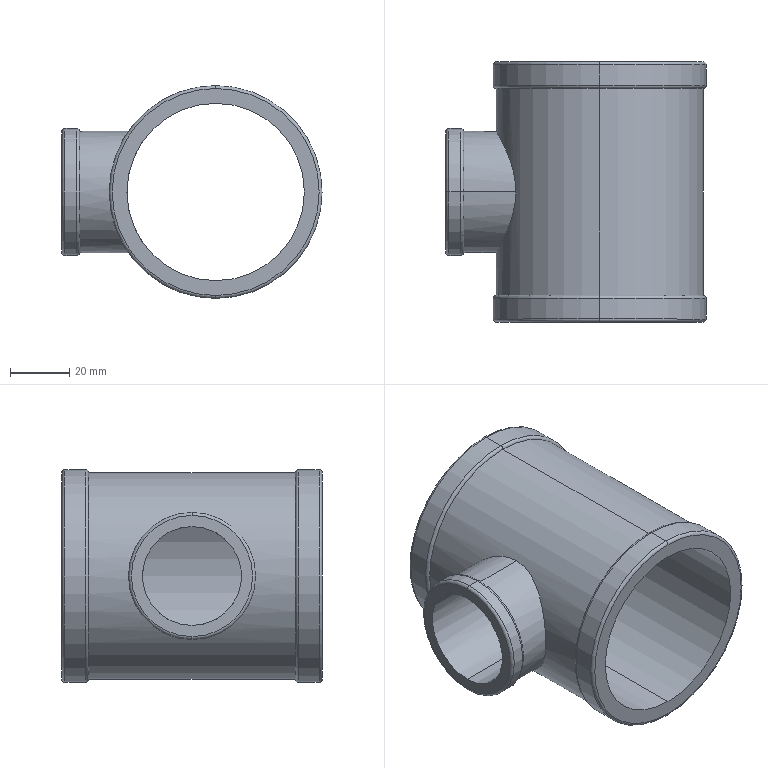Part | SolidWorks | features BossThin 3, Cut 2, Revolution 2, Fillet 1 | 1 solid | 29 faces | box 88 x 88 x 72 mm | volume 98463 mm3 | cylinder 14 | torus 12 | plane 3 | commonest cylinder face diameters 72 x4 33.5 x2 41 x2 43 x2 60 x2 70 x2
STEP:
#1=CARTESIAN_POINT('',(-51.,0.,-21.5));
#2=VERTEX_POINT('',#1);
#3=CARTESIAN_POINT('',(-51.,0.,21.5));
#4=VERTEX_POINT('',#3);
#5=CARTESIAN_POINT('',(-51.,0.,0.));
#6=DIRECTION('',(1.,0.,0.));
#7=DIRECTION('',(0.,0.,1.));
#8=AXIS2_PLACEMENT_3D('',#5,#6,#7);
#9=CIRCLE('',#8,21.5);
#10=EDGE_CURVE('',#2,#4,#9,.T.);
#11=ORIENTED_EDGE('',*,*,#10,.F.);
#12=CARTESIAN_POINT('',(-52.,0.,-20.5));
#13=VERTEX_POINT('',#12);
#14=CARTESIAN_POINT('',(-51.,0.,-20.5));
#15=DIRECTION('',(0.,1.,0.));
#16=DIRECTION('',(0.,0.,1.));
#17=AXIS2_PLACEMENT_3D('',#14,#15,#16);
#18=CIRCLE('',#17,1.);
#19=EDGE_CURVE('',#2,#13,#18,.T.);
#20=ORIENTED_EDGE('',*,*,#19,.T.);
#21=CARTESIAN_POINT('',(-52.,0.,20.5));
#22=VERTEX_POINT('',#21);
#23=CARTESIAN_POINT('',(-52.,0.,0.));
#24=DIRECTION('',(-1.,0.,0.));
#25=DIRECTION('',(0.,0.,1.));
#26=AXIS2_PLACEMENT_3D('',#23,#24,#25);
#27=CIRCLE('',#26,20.5);
#28=EDGE_CURVE('',#22,#13,#27,.T.);
#29=ORIENTED_EDGE('',*,*,#28,.F.);
#30=CARTESIAN_POINT('',(-51.,0.,20.5));
#31=DIRECTION('',(0.,-1.,0.));
#32=DIRECTION('',(0.,0.,-1.));
#33=AXIS2_PLACEMENT_3D('',#30,#31,#32);
#34=CIRCLE('',#33,1.);
#35=EDGE_CURVE('',#4,#22,#34,.T.);
#36=ORIENTED_EDGE('',*,*,#35,.F.);
#37=EDGE_LOOP('',(#11,#20,#29,#36));
#38=FACE_OUTER_BOUND('',#37,.T.);
#39=CARTESIAN_POINT('',(-51.,0.,0.));
#40=DIRECTION('',(-1.,0.,0.));
#41=DIRECTION('',(0.,0.,1.));
#42=AXIS2_PLACEMENT_3D('',#39,#40,#41);
#43=TOROIDAL_SURFACE('',#42,20.5,1.);
#44=ADVANCED_FACE('',(#38),#43,.T.);
#45=CARTESIAN_POINT('',(-46.,0.,20.5));
#46=VERTEX_POINT('',#45);
#47=CARTESIAN_POINT('',(-46.,0.,-20.5));
#48=VERTEX_POINT('',#47);
#49=CARTESIAN_POINT('',(-46.,0.,0.));
#50=DIRECTION('',(-1.,0.,0.));
#51=DIRECTION('',(0.,0.,1.));
#52=AXIS2_PLACEMENT_3D('',#49,#50,#51);
#53=CIRCLE('',#52,20.5);
#54=EDGE_CURVE('',#46,#48,#53,.T.);
#55=ORIENTED_EDGE('',*,*,#54,.T.);
#56=CARTESIAN_POINT('',(-47.,0.,-21.5));
#57=VERTEX_POINT('',#56);
#58=CARTESIAN_POINT('',(-47.,0.,-20.5));
#59=DIRECTION('',(0.,1.,0.));
#60=DIRECTION('',(0.,0.,1.));
#61=AXIS2_PLACEMENT_3D('',#58,#59,#60);
#62=CIRCLE('',#61,1.);
#63=EDGE_CURVE('',#48,#57,#62,.T.);
#64=ORIENTED_EDGE('',*,*,#63,.T.);
#65=CARTESIAN_POINT('',(-47.,0.,21.5));
#66=VERTEX_POINT('',#65);
#67=CARTESIAN_POINT('',(-47.,0.,0.));
#68=DIRECTION('',(-1.,0.,0.));
#69=DIRECTION('',(0.,0.,1.));
#70=AXIS2_PLACEMENT_3D('',#67,#68,#69);
#71=CIRCLE('',#70,21.5);
#72=EDGE_CURVE('',#66,#57,#71,.T.);
#73=ORIENTED_EDGE('',*,*,#72,.F.);
#74=CARTESIAN_POINT('',(-47.,0.,20.5));
#75=DIRECTION('',(0.,-1.,0.));
#76=DIRECTION('',(0.,0.,-1.));
#77=AXIS2_PLACEMENT_3D('',#74,#75,#76);
#78=CIRCLE('',#77,1.);
#79=EDGE_CURVE('',#46,#66,#78,.T.);
#80=ORIENTED_EDGE('',*,*,#79,.F.);
#81=EDGE_LOOP('',(#55,#64,#73,#80));
#82=FACE_OUTER_BOUND('',#81,.T.);
#83=CARTESIAN_POINT('',(-47.,0.,0.));
#84=DIRECTION('',(-1.,0.,0.));
#85=DIRECTION('',(0.,0.,1.));
#86=AXIS2_PLACEMENT_3D('',#83,#84,#85);
#87=TOROIDAL_SURFACE('',#86,20.5,1.);
#88=ADVANCED_FACE('',(#82),#87,.T.);
#89=CARTESIAN_POINT('',(0.,44.,35.));
#90=VERTEX_POINT('',#89);
#91=CARTESIAN_POINT('',(0.,44.,-35.));
#92=VERTEX_POINT('',#91);
#93=CARTESIAN_POINT('',(0.,44.,0.));
#94=DIRECTION('',(0.,1.,0.));
#95=DIRECTION('',(0.,0.,-1.));
#96=AXIS2_PLACEMENT_3D('',#93,#94,#95);
#97=CIRCLE('',#96,35.);
#98=EDGE_CURVE('',#90,#92,#97,.T.);
#99=ORIENTED_EDGE('',*,*,#98,.F.);
#100=CARTESIAN_POINT('',(0.,43.,36.));
#101=VERTEX_POINT('',#100);
#102=CARTESIAN_POINT('',(0.,43.,35.));
#103=DIRECTION('',(1.,0.,0.));
#104=DIRECTION('',(0.,0.,-1.));
#105=AXIS2_PLACEMENT_3D('',#102,#103,#104);
#106=CIRCLE('',#105,1.);
#107=EDGE_CURVE('',#90,#101,#106,.T.);
#108=ORIENTED_EDGE('',*,*,#107,.T.);
#109=CARTESIAN_POINT('',(0.,43.,-36.));
#110=VERTEX_POINT('',#109);
#111=CARTESIAN_POINT('',(0.,43.,0.));
#112=DIRECTION('',(0.,-1.,0.));
#113=DIRECTION('',(0.,0.,-1.));
#114=AXIS2_PLACEMENT_3D('',#111,#112,#113);
#115=CIRCLE('',#114,36.);
#116=EDGE_CURVE('',#110,#101,#115,.T.);
#117=ORIENTED_EDGE('',*,*,#116,.F.);
#118=CARTESIAN_POINT('',(0.,43.,-35.));
#119=DIRECTION('',(-1.,0.,0.));
#120=DIRECTION('',(0.,0.,1.));
#121=AXIS2_PLACEMENT_3D('',#118,#119,#120);
#122=CIRCLE('',#121,1.);
#123=EDGE_CURVE('',#92,#110,#122,.T.);
#124=ORIENTED_EDGE('',*,*,#123,.F.);
#125=EDGE_LOOP('',(#99,#108,#117,#124));
#126=FACE_OUTER_BOUND('',#125,.T.);
#127=CARTESIAN_POINT('',(0.,43.,0.));
#128=DIRECTION('',(0.,-1.,0.));
#129=DIRECTION('',(0.,0.,-1.));
#130=AXIS2_PLACEMENT_3D('',#127,#128,#129);
#131=TOROIDAL_SURFACE('',#130,35.,1.);
#132=ADVANCED_FACE('',(#126),#131,.T.);
#133=CARTESIAN_POINT('',(0.,35.,35.));
#134=VERTEX_POINT('',#133);
#135=CARTESIAN_POINT('',(0.,35.,-35.));
#136=VERTEX_POINT('',#135);
#137=CARTESIAN_POINT('',(0.,35.,0.));
#138=DIRECTION('',(0.,1.,0.));
#139=DIRECTION('',(0.,0.,1.));
#140=AXIS2_PLACEMENT_3D('',#137,#138,#139);
#141=CIRCLE('',#140,35.);
#142=EDGE_CURVE('',#134,#136,#141,.T.);
#143=ORIENTED_EDGE('',*,*,#142,.T.);
#144=CARTESIAN_POINT('',(0.,36.,-36.));
#145=VERTEX_POINT('',#144);
#146=CARTESIAN_POINT('',(0.,36.,-35.));
#147=DIRECTION('',(1.,0.,0.));
#148=DIRECTION('',(0.,0.,-1.));
#149=AXIS2_PLACEMENT_3D('',#146,#147,#148);
#150=CIRCLE('',#149,1.);
#151=EDGE_CURVE('',#136,#145,#150,.T.);
#152=ORIENTED_EDGE('',*,*,#151,.T.);
#153=CARTESIAN_POINT('',(0.,36.,36.));
#154=VERTEX_POINT('',#153);
#155=CARTESIAN_POINT('',(0.,36.,0.));
#156=DIRECTION('',(0.,1.,0.));
#157=DIRECTION('',(0.,0.,1.));
#158=AXIS2_PLACEMENT_3D('',#155,#156,#157);
#159=CIRCLE('',#158,36.);
#160=EDGE_CURVE('',#154,#145,#159,.T.);
#161=ORIENTED_EDGE('',*,*,#160,.F.);
#162=CARTESIAN_POINT('',(0.,36.,35.));
#163=DIRECTION('',(-1.,0.,0.));
#164=DIRECTION('',(0.,0.,1.));
#165=AXIS2_PLACEMENT_3D('',#162,#163,#164);
#166=CIRCLE('',#165,1.);
#167=EDGE_CURVE('',#134,#154,#166,.T.);
#168=ORIENTED_EDGE('',*,*,#167,.F.);
#169=EDGE_LOOP('',(#143,#152,#161,#168));
#170=FACE_OUTER_BOUND('',#169,.T.);
#171=CARTESIAN_POINT('',(0.,36.,0.));
#172=DIRECTION('',(0.,1.,0.));
#173=DIRECTION('',(0.,0.,1.));
#174=AXIS2_PLACEMENT_3D('',#171,#172,#173);
#175=TOROIDAL_SURFACE('',#174,35.,1.);
#176=ADVANCED_FACE('',(#170),#175,.T.);
#177=CARTESIAN_POINT('',(0.,-35.,-35.));
#178=VERTEX_POINT('',#177);
#179=CARTESIAN_POINT('',(0.,-35.,35.));
#180=VERTEX_POINT('',#179);
#181=CARTESIAN_POINT('',(0.,-35.,0.));
#182=DIRECTION('',(0.,-1.,0.));
#183=DIRECTION('',(0.,0.,-1.));
#184=AXIS2_PLACEMENT_3D('',#181,#182,#183);
#185=CIRCLE('',#184,35.);
#186=EDGE_CURVE('',#178,#180,#185,.T.);
#187=ORIENTED_EDGE('',*,*,#186,.T.);
#188=CARTESIAN_POINT('',(0.,-36.,36.));
#189=VERTEX_POINT('',#188);
#190=CARTESIAN_POINT('',(0.,-36.,35.));
#191=DIRECTION('',(1.,0.,0.));
#192=DIRECTION('',(0.,0.,-1.));
#193=AXIS2_PLACEMENT_3D('',#190,#191,#192);
#194=CIRCLE('',#193,1.);
#195=EDGE_CURVE('',#180,#189,#194,.T.);
#196=ORIENTED_EDGE('',*,*,#195,.T.);
#197=CARTESIAN_POINT('',(0.,-36.,-36.));
#198=VERTEX_POINT('',#197);
#199=CARTESIAN_POINT('',(0.,-36.,0.));
#200=DIRECTION('',(0.,-1.,0.));
#201=DIRECTION('',(0.,0.,-1.));
#202=AXIS2_PLACEMENT_3D('',#199,#200,#201);
#203=CIRCLE('',#202,36.);
#204=EDGE_CURVE('',#198,#189,#203,.T.);
#205=ORIENTED_EDGE('',*,*,#204,.F.);
#206=CARTESIAN_POINT('',(0.,-36.,-35.));
#207=DIRECTION('',(-1.,0.,0.));
#208=DIRECTION('',(0.,0.,1.));
#209=AXIS2_PLACEMENT_3D('',#206,#207,#208);
#210=CIRCLE('',#209,1.);
#211=EDGE_CURVE('',#178,#198,#210,.T.);
#212=ORIENTED_EDGE('',*,*,#211,.F.);
#213=EDGE_LOOP('',(#187,#196,#205,#212));
#214=FACE_OUTER_BOUND('',#213,.T.);
#215=CARTESIAN_POINT('',(0.,-36.,0.));
#216=DIRECTION('',(0.,-1.,0.));
#217=DIRECTION('',(0.,0.,-1.));
#218=AXIS2_PLACEMENT_3D('',#215,#216,#217);
#219=TOROIDAL_SURFACE('',#218,35.,1.);
#220=ADVANCED_FACE('',(#214),#219,.T.);
#221=CARTESIAN_POINT('',(0.,-44.,-35.));
#222=VERTEX_POINT('',#221);
#223=CARTESIAN_POINT('',(0.,-44.,35.));
#224=VERTEX_POINT('',#223);
#225=CARTESIAN_POINT('',(0.,-44.,0.));
#226=DIRECTION('',(0.,-1.,0.));
#227=DIRECTION('',(0.,0.,1.));
#228=AXIS2_PLACEMENT_3D('',#225,#226,#227);
#229=CIRCLE('',#228,35.);
#230=EDGE_CURVE('',#222,#224,#229,.T.);
#231=ORIENTED_EDGE('',*,*,#230,.F.);
#232=CARTESIAN_POINT('',(0.,-43.,-36.));
#233=VERTEX_POINT('',#232);
#234=CARTESIAN_POINT('',(0.,-43.,-35.));
#235=DIRECTION('',(1.,0.,0.));
#236=DIRECTION('',(0.,0.,-1.));
#237=AXIS2_PLACEMENT_3D('',#234,#235,#236);
#238=CIRCLE('',#237,1.);
#239=EDGE_CURVE('',#222,#233,#238,.T.);
#240=ORIENTED_EDGE('',*,*,#239,.T.);
#241=CARTESIAN_POINT('',(0.,-43.,36.));
#242=VERTEX_POINT('',#241);
#243=CARTESIAN_POINT('',(0.,-43.,0.));
#244=DIRECTION('',(0.,1.,0.));
#245=DIRECTION('',(0.,0.,1.));
#246=AXIS2_PLACEMENT_3D('',#243,#244,#245);
#247=CIRCLE('',#246,36.);
#248=EDGE_CURVE('',#242,#233,#247,.T.);
#249=ORIENTED_EDGE('',*,*,#248,.F.);
#250=CARTESIAN_POINT('',(0.,-43.,35.));
#251=DIRECTION('',(-1.,0.,0.));
#252=DIRECTION('',(0.,0.,1.));
#253=AXIS2_PLACEMENT_3D('',#250,#251,#252);
#254=CIRCLE('',#253,1.);
#255=EDGE_CURVE('',#224,#242,#254,.T.);
#256=ORIENTED_EDGE('',*,*,#255,.F.);
#257=EDGE_LOOP('',(#231,#240,#249,#256));
#258=FACE_OUTER_BOUND('',#257,.T.);
#259=CARTESIAN_POINT('',(0.,-43.,0.));
#260=DIRECTION('',(0.,1.,0.));
#261=DIRECTION('',(0.,0.,1.));
#262=AXIS2_PLACEMENT_3D('',#259,#260,#261);
#263=TOROIDAL_SURFACE('',#262,35.,1.);
#264=ADVANCED_FACE('',(#258),#263,.T.);
#265=ORIENTED_EDGE('',*,*,#72,.T.);
#266=CARTESIAN_POINT('',(-46.,0.,-21.5));
#267=DIRECTION('',(-1.,0.,0.));
#268=VECTOR('',#267,1000.);
#269=LINE('',#266,#268);
#270=EDGE_CURVE('',#57,#2,#269,.T.);
#271=ORIENTED_EDGE('',*,*,#270,.T.);
#272=ORIENTED_EDGE('',*,*,#10,.T.);
#273=CARTESIAN_POINT('',(-46.,0.,21.5));
#274=DIRECTION('',(-1.,0.,0.));
#275=VECTOR('',#274,1000.);
#276=LINE('',#273,#275);
#277=EDGE_CURVE('',#66,#4,#276,.T.);
#278=ORIENTED_EDGE('',*,*,#277,.F.);
#279=EDGE_LOOP('',(#265,#271,#272,#278));
#280=FACE_OUTER_BOUND('',#279,.T.);
#281=CARTESIAN_POINT('',(-46.,0.,0.));
#282=DIRECTION('',(-1.,0.,0.));
#283=DIRECTION('',(0.,0.,1.));
#284=AXIS2_PLACEMENT_3D('',#281,#282,#283);
#285=CYLINDRICAL_SURFACE('',#284,21.5);
#286=ADVANCED_FACE('',(#280),#285,.T.);
#287=ORIENTED_EDGE('',*,*,#160,.T.);
#288=CARTESIAN_POINT('',(0.,35.,-36.));
#289=DIRECTION('',(0.,1.,0.));
#290=VECTOR('',#289,1000.);
#291=LINE('',#288,#290);
#292=EDGE_CURVE('',#145,#110,#291,.T.);
#293=ORIENTED_EDGE('',*,*,#292,.T.);
#294=ORIENTED_EDGE('',*,*,#116,.T.);
#295=CARTESIAN_POINT('',(0.,35.,36.));
#296=DIRECTION('',(0.,1.,0.));
#297=VECTOR('',#296,1000.);
#298=LINE('',#295,#297);
#299=EDGE_CURVE('',#154,#101,#298,.T.);
#300=ORIENTED_EDGE('',*,*,#299,.F.);
#301=EDGE_LOOP('',(#287,#293,#294,#300));
#302=FACE_OUTER_BOUND('',#301,.T.);
#303=CARTESIAN_POINT('',(0.,35.,0.));
#304=DIRECTION('',(0.,1.,0.));
#305=DIRECTION('',(0.,0.,1.));
#306=AXIS2_PLACEMENT_3D('',#303,#304,#305);
#307=CYLINDRICAL_SURFACE('',#306,36.);
#308=ADVANCED_FACE('',(#302),#307,.T.);
#309=ORIENTED_EDGE('',*,*,#204,.T.);
#310=CARTESIAN_POINT('',(0.,-35.,36.));
#311=DIRECTION('',(0.,-1.,0.));
#312=VECTOR('',#311,1000.);
#313=LINE('',#310,#312);
#314=EDGE_CURVE('',#189,#242,#313,.T.);
#315=ORIENTED_EDGE('',*,*,#314,.T.);
#316=ORIENTED_EDGE('',*,*,#248,.T.);
#317=CARTESIAN_POINT('',(0.,-35.,-36.));
#318=DIRECTION('',(0.,-1.,0.));
#319=VECTOR('',#318,1000.);
#320=LINE('',#317,#319);
#321=EDGE_CURVE('',#198,#233,#320,.T.);
#322=ORIENTED_EDGE('',*,*,#321,.F.);
#323=EDGE_LOOP('',(#309,#315,#316,#322));
#324=FACE_OUTER_BOUND('',#323,.T.);
#325=CARTESIAN_POINT('',(0.,-35.,0.));
#326=DIRECTION('',(0.,-1.,0.));
#327=DIRECTION('',(0.,0.,-1.));
#328=AXIS2_PLACEMENT_3D('',#325,#326,#327);
#329=CYLINDRICAL_SURFACE('',#328,36.);
#330=ADVANCED_FACE('',(#324),#329,.T.);
#331=CARTESIAN_POINT('',(-24.889,0.,-16.75));
#332=VERTEX_POINT('',#331);
#333=CARTESIAN_POINT('',(-24.889,0.,16.75));
#334=VERTEX_POINT('',#333);
#335=CARTESIAN_POINT('',(-24.889,0.,-16.75));
#336=CARTESIAN_POINT('',(-24.889,-1.134,-16.75));
#337=CARTESIAN_POINT('',(-24.966,-2.242,-16.636));
#338=CARTESIAN_POINT('',(-25.182,-3.871,-16.306));
#339=CARTESIAN_POINT('',(-25.27,-4.408,-16.169));
#340=CARTESIAN_POINT('',(-25.477,-5.471,-15.841));
#341=CARTESIAN_POINT('',(-25.594,-5.989,-15.652));
#342=CARTESIAN_POINT('',(-25.975,-7.498,-15.018));
#343=CARTESIAN_POINT('',(-26.27,-8.448,-14.504));
#344=CARTESIAN_POINT('',(-26.744,-9.798,-13.596));
#345=CARTESIAN_POINT('',(-26.907,-10.231,-13.273));
#346=CARTESIAN_POINT('',(-27.232,-11.059,-12.592));
#347=CARTESIAN_POINT('',(-27.396,-11.455,-12.233));
#348=CARTESIAN_POINT('',(-27.721,-12.212,-11.477));
#349=CARTESIAN_POINT('',(-27.882,-12.573,-11.08));
#350=CARTESIAN_POINT('',(-28.199,-13.26,-10.248));
#351=CARTESIAN_POINT('',(-28.354,-13.587,-9.811));
#352=CARTESIAN_POINT('',(-28.797,-14.495,-8.464));
#353=CARTESIAN_POINT('',(-29.062,-15.01,-7.514));
#354=CARTESIAN_POINT('',(-29.398,-15.647,-6.003));
#355=CARTESIAN_POINT('',(-29.499,-15.836,-5.485));
#356=CARTESIAN_POINT('',(-29.678,-16.166,-4.419));
#357=CARTESIAN_POINT('',(-29.754,-16.305,-3.876));
#358=CARTESIAN_POINT('',(-29.936,-16.636,-2.243));
#359=CARTESIAN_POINT('',(-30.,-16.749,-1.137));
#360=CARTESIAN_POINT('',(-30.,-16.75,0.549));
#361=CARTESIAN_POINT('',(-29.984,-16.722,1.118));
#362=CARTESIAN_POINT('',(-29.922,-16.61,2.235));
#363=CARTESIAN_POINT('',(-29.875,-16.526,2.786));
#364=CARTESIAN_POINT('',(-29.754,-16.305,3.875));
#365=CARTESIAN_POINT('',(-29.679,-16.168,4.413));
#366=CARTESIAN_POINT('',(-29.501,-15.84,5.475));
#367=CARTESIAN_POINT('',(-29.398,-15.648,6.001));
#368=CARTESIAN_POINT('',(-29.06,-15.006,7.524));
#369=CARTESIAN_POINT('',(-28.793,-14.486,8.479));
#370=CARTESIAN_POINT('',(-28.348,-13.574,9.829));
#371=CARTESIAN_POINT('',(-28.192,-13.246,10.266));
#372=CARTESIAN_POINT('',(-27.876,-12.558,11.097));
#373=CARTESIAN_POINT('',(-27.714,-12.197,11.493));
#374=CARTESIAN_POINT('',(-27.389,-11.438,12.248));
#375=CARTESIAN_POINT('',(-27.225,-11.041,12.607));
#376=CARTESIAN_POINT('',(-26.899,-10.211,13.288));
#377=CARTESIAN_POINT('',(-26.736,-9.776,13.612));
#378=CARTESIAN_POINT('',(-26.263,-8.427,14.516));
#379=CARTESIAN_POINT('',(-25.97,-7.478,15.027));
#380=CARTESIAN_POINT('',(-25.591,-5.977,15.657));
#381=CARTESIAN_POINT('',(-25.476,-5.463,15.844));
#382=CARTESIAN_POINT('',(-25.27,-4.406,16.17));
#383=CARTESIAN_POINT('',(-25.18,-3.86,16.309));
#384=CARTESIAN_POINT('',(-24.964,-2.223,16.639));
#385=CARTESIAN_POINT('',(-24.889,-1.119,16.75));
#386=CARTESIAN_POINT('',(-24.889,0.,16.75));
#387=B_SPLINE_CURVE_WITH_KNOTS('',3,(#335,#336,#337,#338,#339,#340,#341,#342,#343,#344,#345,#346,#347,#348,#349,#350,#351,#352,#353,#354,#355,#356,#357,#358,#359,#360,#361,#362,#363,#364,#365,#366,#367,#368,#369,#370,#371,#372,#373,#374,#375,#376,#377,#378,#379,#380,#381,#382,#383,#384,#385,#386),.UNSPECIFIED.,.F.,.F.,(4,2,2,2,2,2,2,2,2,2,2,2,2,2,2,2,2,2,2,2,2,2,2,2,2,4),(0.,0.003346,0.005019,0.006692,0.01004,0.01171,0.01338,0.01506,0.01673,0.02007,0.02175,0.02342,0.02677,0.02844,0.03011,0.03179,0.03346,0.0368,0.03848,0.04015,0.04182,0.0435,0.04684,0.04851,0.05019,0.05353),.UNSPECIFIED.);
#388=EDGE_CURVE('',#332,#334,#387,.T.);
#389=ORIENTED_EDGE('',*,*,#388,.T.);
#390=CARTESIAN_POINT('',(-24.889,0.,16.75));
#391=CARTESIAN_POINT('',(-24.889,0.2789,16.75));
#392=CARTESIAN_POINT('',(-24.893,0.5586,16.743));
#393=CARTESIAN_POINT('',(-24.912,1.12,16.715));
#394=CARTESIAN_POINT('',(-24.926,1.403,16.694));
#395=CARTESIAN_POINT('',(-24.983,2.243,16.609));
#396=CARTESIAN_POINT('',(-25.039,2.794,16.525));
#397=CARTESIAN_POINT('',(-25.183,3.88,16.304));
#398=CARTESIAN_POINT('',(-25.272,4.414,16.167));
#399=CARTESIAN_POINT('',(-25.477,5.468,15.842));
#400=CARTESIAN_POINT('',(-25.594,5.989,15.652));
#401=CARTESIAN_POINT('',(-25.977,7.505,15.014));
#402=CARTESIAN_POINT('',(-26.272,8.454,14.5));
#403=CARTESIAN_POINT('',(-26.744,9.796,13.598));
#404=CARTESIAN_POINT('',(-26.907,10.231,13.273));
#405=CARTESIAN_POINT('',(-27.233,11.062,12.589));
#406=CARTESIAN_POINT('',(-27.397,11.458,12.23));
#407=CARTESIAN_POINT('',(-27.884,12.592,11.098));
#408=CARTESIAN_POINT('',(-28.202,13.275,10.272));
#409=CARTESIAN_POINT('',(-28.648,14.189,8.918));
#410=CARTESIAN_POINT('',(-28.789,14.471,8.452));
#411=CARTESIAN_POINT('',(-29.052,14.988,7.498));
#412=CARTESIAN_POINT('',(-29.174,15.223,7.009));
#413=CARTESIAN_POINT('',(-29.397,15.646,6.006));
#414=CARTESIAN_POINT('',(-29.498,15.834,5.491));
#415=CARTESIAN_POINT('',(-29.631,16.079,4.7));
#416=CARTESIAN_POINT('',(-29.672,16.155,4.433));
#417=CARTESIAN_POINT('',(-29.748,16.294,3.892));
#418=CARTESIAN_POINT('',(-29.782,16.357,3.618));
#419=CARTESIAN_POINT('',(-29.936,16.636,2.246));
#420=CARTESIAN_POINT('',(-29.999,16.748,1.139));
#421=CARTESIAN_POINT('',(-30.,16.751,-0.5347));
#422=CARTESIAN_POINT('',(-29.985,16.724,-1.095));
#423=CARTESIAN_POINT('',(-29.923,16.612,-2.221));
#424=CARTESIAN_POINT('',(-29.876,16.528,-2.774));
#425=CARTESIAN_POINT('',(-29.694,16.197,-4.41));
#426=CARTESIAN_POINT('',(-29.516,15.871,-5.468));
#427=CARTESIAN_POINT('',(-29.063,15.012,-7.511));
#428=CARTESIAN_POINT('',(-28.796,14.493,-8.466));
#429=CARTESIAN_POINT('',(-28.207,13.285,-10.259));
#430=CARTESIAN_POINT('',(-27.883,12.589,-11.101));
#431=CARTESIAN_POINT('',(-27.232,11.073,-12.613));
#432=CARTESIAN_POINT('',(-26.903,10.249,-13.293));
#433=CARTESIAN_POINT('',(-26.43,8.905,-14.197));
#434=CARTESIAN_POINT('',(-26.276,8.437,-14.48));
#435=CARTESIAN_POINT('',(-25.986,7.485,-14.994));
#436=CARTESIAN_POINT('',(-25.849,6.997,-15.228));
#437=CARTESIAN_POINT('',(-25.471,5.499,-15.859));
#438=CARTESIAN_POINT('',(-25.261,4.455,-16.186));
#439=CARTESIAN_POINT('',(-24.967,2.255,-16.635));
#440=CARTESIAN_POINT('',(-24.889,1.131,-16.75));
#441=CARTESIAN_POINT('',(-24.889,0.,-16.75));
#442=B_SPLINE_CURVE_WITH_KNOTS('',3,(#390,#391,#392,#393,#394,#395,#396,#397,#398,#399,#400,#401,#402,#403,#404,#405,#406,#407,#408,#409,#410,#411,#412,#413,#414,#415,#416,#417,#418,#419,#420,#421,#422,#423,#424,#425,#426,#427,#428,#429,#430,#431,#432,#433,#434,#435,#436,#437,#438,#439,#440,#441),.UNSPECIFIED.,.F.,.F.,(4,2,2,2,2,2,2,2,2,2,2,2,2,2,2,2,2,2,2,2,2,2,2,2,2,4),(0.05353,0.05437,0.0552,0.05687,0.05854,0.06021,0.06354,0.06521,0.06688,0.07022,0.07189,0.07355,0.07522,0.07606,0.07689,0.08023,0.0819,0.08356,0.0869,0.09024,0.09358,0.09691,0.09858,0.1002,0.1036,0.1069),.UNSPECIFIED.);
#443=EDGE_CURVE('',#334,#332,#442,.T.);
#444=ORIENTED_EDGE('',*,*,#443,.T.);
#445=EDGE_LOOP('',(#389,#444));
#446=FACE_BOUND('',#445,.T.);
#447=CARTESIAN_POINT('',(0.,44.,30.));
#448=VERTEX_POINT('',#447);
#449=CARTESIAN_POINT('',(0.,44.,-30.));
#450=VERTEX_POINT('',#449);
#451=CARTESIAN_POINT('',(0.,44.,0.));
#452=DIRECTION('',(0.,-1.,0.));
#453=DIRECTION('',(0.,0.,-1.));
#454=AXIS2_PLACEMENT_3D('',#451,#452,#453);
#455=CIRCLE('',#454,30.);
#456=EDGE_CURVE('',#448,#450,#455,.T.);
#457=ORIENTED_EDGE('',*,*,#456,.F.);
#458=CARTESIAN_POINT('',(0.,-44.,30.));
#459=VERTEX_POINT('',#458);
#460=CARTESIAN_POINT('',(0.,0.,30.));
#461=DIRECTION('',(0.,-1.,0.));
#462=VECTOR('',#461,1000.);
#463=LINE('',#460,#462);
#464=EDGE_CURVE('',#448,#459,#463,.T.);
#465=ORIENTED_EDGE('',*,*,#464,.T.);
#466=CARTESIAN_POINT('',(0.,-44.,-30.));
#467=VERTEX_POINT('',#466);
#468=CARTESIAN_POINT('',(0.,-44.,0.));
#469=DIRECTION('',(0.,-1.,0.));
#470=DIRECTION('',(0.,0.,-1.));
#471=AXIS2_PLACEMENT_3D('',#468,#469,#470);
#472=CIRCLE('',#471,30.);
#473=EDGE_CURVE('',#459,#467,#472,.T.);
#474=ORIENTED_EDGE('',*,*,#473,.T.);
#475=CARTESIAN_POINT('',(0.,0.,-30.));
#476=DIRECTION('',(0.,-1.,0.));
#477=VECTOR('',#476,1000.);
#478=LINE('',#475,#477);
#479=EDGE_CURVE('',#450,#467,#478,.T.);
#480=ORIENTED_EDGE('',*,*,#479,.F.);
#481=EDGE_LOOP('',(#457,#465,#474,#480));
#482=FACE_OUTER_BOUND('',#481,.T.);
#483=CARTESIAN_POINT('',(0.,0.,0.));
#484=DIRECTION('',(0.,-1.,0.));
#485=DIRECTION('',(0.,0.,-1.));
#486=AXIS2_PLACEMENT_3D('',#483,#484,#485);
#487=CYLINDRICAL_SURFACE('',#486,30.);
#488=ADVANCED_FACE('',(#446,#482),#487,.F.);
#489=CARTESIAN_POINT('',(-52.,0.,16.75));
#490=VERTEX_POINT('',#489);
#491=CARTESIAN_POINT('',(-52.,0.,-16.75));
#492=VERTEX_POINT('',#491);
#493=CARTESIAN_POINT('',(-52.,0.,0.));
#494=DIRECTION('',(1.,0.,0.));
#495=DIRECTION('',(0.,0.,-1.));
#496=AXIS2_PLACEMENT_3D('',#493,#494,#495);
#497=CIRCLE('',#496,16.75);
#498=EDGE_CURVE('',#490,#492,#497,.T.);
#499=ORIENTED_EDGE('',*,*,#498,.F.);
#500=CARTESIAN_POINT('',(0.,0.,16.75));
#501=DIRECTION('',(1.,0.,0.));
#502=VECTOR('',#501,1000.);
#503=LINE('',#500,#502);
#504=EDGE_CURVE('',#490,#334,#503,.T.);
#505=ORIENTED_EDGE('',*,*,#504,.T.);
#506=ORIENTED_EDGE('',*,*,#388,.F.);
#507=CARTESIAN_POINT('',(0.,0.,-16.75));
#508=DIRECTION('',(1.,0.,0.));
#509=VECTOR('',#508,1000.);
#510=LINE('',#507,#509);
#511=EDGE_CURVE('',#492,#332,#510,.T.);
#512=ORIENTED_EDGE('',*,*,#511,.F.);
#513=EDGE_LOOP('',(#499,#505,#506,#512));
#514=FACE_OUTER_BOUND('',#513,.T.);
#515=CARTESIAN_POINT('',(0.,0.,0.));
#516=DIRECTION('',(1.,0.,0.));
#517=DIRECTION('',(0.,0.,-1.));
#518=AXIS2_PLACEMENT_3D('',#515,#516,#517);
#519=CYLINDRICAL_SURFACE('',#518,16.75);
#520=ADVANCED_FACE('',(#514),#519,.F.);
#521=ORIENTED_EDGE('',*,*,#142,.F.);
#522=CARTESIAN_POINT('',(0.,0.,35.));
#523=DIRECTION('',(0.,-1.,0.));
#524=VECTOR('',#523,1000.);
#525=LINE('',#522,#524);
#526=EDGE_CURVE('',#134,#180,#525,.T.);
#527=ORIENTED_EDGE('',*,*,#526,.T.);
#528=ORIENTED_EDGE('',*,*,#186,.F.);
#529=CARTESIAN_POINT('',(0.,0.,-35.));
#530=DIRECTION('',(0.,-1.,0.));
#531=VECTOR('',#530,1000.);
#532=LINE('',#529,#531);
#533=EDGE_CURVE('',#136,#178,#532,.T.);
#534=ORIENTED_EDGE('',*,*,#533,.F.);
#535=EDGE_LOOP('',(#521,#527,#528,#534));
#536=FACE_OUTER_BOUND('',#535,.T.);
#537=CARTESIAN_POINT('',(0.,0.,0.));
#538=DIRECTION('',(0.,-1.,0.));
#539=DIRECTION('',(0.,0.,-1.));
#540=AXIS2_PLACEMENT_3D('',#537,#538,#539);
#541=CYLINDRICAL_SURFACE('',#540,35.);
#542=ADVANCED_FACE('',(#536),#541,.T.);
#543=ORIENTED_EDGE('',*,*,#54,.F.);
#544=CARTESIAN_POINT('',(-28.368,0.,20.5));
#545=VERTEX_POINT('',#544);
#546=CARTESIAN_POINT('',(0.,0.,20.5));
#547=DIRECTION('',(1.,0.,0.));
#548=VECTOR('',#547,1000.);
#549=LINE('',#546,#548);
#550=EDGE_CURVE('',#46,#545,#549,.T.);
#551=ORIENTED_EDGE('',*,*,#550,.T.);
#552=CARTESIAN_POINT('',(-28.368,0.,-20.5));
#553=VERTEX_POINT('',#552);
#554=CARTESIAN_POINT('',(-28.368,0.,-20.5));
#555=CARTESIAN_POINT('',(-28.368,1.391,-20.5));
#556=CARTESIAN_POINT('',(-28.471,2.75,-20.36));
#557=CARTESIAN_POINT('',(-28.755,4.745,-19.955));
#558=CARTESIAN_POINT('',(-28.871,5.403,-19.787));
#559=CARTESIAN_POINT('',(-29.143,6.704,-19.385));
#560=CARTESIAN_POINT('',(-29.295,7.336,-19.154));
#561=CARTESIAN_POINT('',(-29.793,9.18,-18.378));
#562=CARTESIAN_POINT('',(-30.177,10.341,-17.75));
#563=CARTESIAN_POINT('',(-30.999,12.54,-16.272));
#564=CARTESIAN_POINT('',(-31.426,13.547,-15.441));
#565=CARTESIAN_POINT('',(-32.057,14.935,-14.058));
#566=CARTESIAN_POINT('',(-32.265,15.376,-13.574));
#567=CARTESIAN_POINT('',(-32.674,16.217,-12.558));
#568=CARTESIAN_POINT('',(-32.875,16.616,-12.025));
#569=CARTESIAN_POINT('',(-33.445,17.726,-10.383));
#570=CARTESIAN_POINT('',(-33.787,18.357,-9.222));
#571=CARTESIAN_POINT('',(-34.22,19.14,-7.374));
#572=CARTESIAN_POINT('',(-34.351,19.373,-6.74));
#573=CARTESIAN_POINT('',(-34.582,19.779,-5.432));
#574=CARTESIAN_POINT('',(-34.68,19.949,-4.77));
#575=CARTESIAN_POINT('',(-34.916,20.358,-2.77));
#576=CARTESIAN_POINT('',(-34.999,20.498,-1.414));
#577=CARTESIAN_POINT('',(-35.001,20.501,0.6562));
#578=CARTESIAN_POINT('',(-34.981,20.467,1.354));
#579=CARTESIAN_POINT('',(-34.901,20.33,2.723));
#580=CARTESIAN_POINT('',(-34.841,20.228,3.399));
#581=CARTESIAN_POINT('',(-34.685,19.957,4.735));
#582=CARTESIAN_POINT('',(-34.588,19.789,5.394));
#583=CARTESIAN_POINT('',(-34.36,19.387,6.697));
#584=CARTESIAN_POINT('',(-34.228,19.153,7.34));
#585=CARTESIAN_POINT('',(-33.792,18.368,9.203));
#586=CARTESIAN_POINT('',(-33.448,17.732,10.372));
#587=CARTESIAN_POINT('',(-32.875,16.616,12.025));
#588=CARTESIAN_POINT('',(-32.674,16.217,12.558));
#589=CARTESIAN_POINT('',(-32.266,15.378,13.572));
#590=CARTESIAN_POINT('',(-32.058,14.937,14.056));
#591=CARTESIAN_POINT('',(-31.637,14.012,14.978));
#592=CARTESIAN_POINT('',(-31.425,13.528,15.417));
#593=CARTESIAN_POINT('',(-31.002,12.514,16.25));
#594=CARTESIAN_POINT('',(-30.791,11.982,16.647));
#595=CARTESIAN_POINT('',(-30.177,10.34,17.75));
#596=CARTESIAN_POINT('',(-29.795,9.185,18.375));
#597=CARTESIAN_POINT('',(-29.299,7.35,19.149));
#598=CARTESIAN_POINT('',(-29.146,6.721,19.379));
#599=CARTESIAN_POINT('',(-28.943,5.749,19.68));
#600=CARTESIAN_POINT('',(-28.879,5.419,19.774));
#601=CARTESIAN_POINT('',(-28.762,4.757,19.943));
#602=CARTESIAN_POINT('',(-28.709,4.424,20.02));
#603=CARTESIAN_POINT('',(-28.471,2.753,20.36));
#604=CARTESIAN_POINT('',(-28.368,1.39,20.5));
#605=CARTESIAN_POINT('',(-28.368,0.,20.5));
#606=B_SPLINE_CURVE_WITH_KNOTS('',3,(#554,#555,#556,#557,#558,#559,#560,#561,#562,#563,#564,#565,#566,#567,#568,#569,#570,#571,#572,#573,#574,#575,#576,#577,#578,#579,#580,#581,#582,#583,#584,#585,#586,#587,#588,#589,#590,#591,#592,#593,#594,#595,#596,#597,#598,#599,#600,#601,#602,#603,#604,#605),.UNSPECIFIED.,.F.,.F.,(4,2,2,2,2,2,2,2,2,2,2,2,2,2,2,2,2,2,2,2,2,2,2,2,2,4),(0.,0.004103,0.006155,0.008207,0.01231,0.01641,0.01847,0.02052,0.02462,0.02667,0.02872,0.03283,0.03488,0.03693,0.03898,0.04103,0.04514,0.04719,0.04924,0.05129,0.05334,0.05745,0.0595,0.06052,0.06155,0.06565),.UNSPECIFIED.);
#607=EDGE_CURVE('',#553,#545,#606,.T.);
#608=ORIENTED_EDGE('',*,*,#607,.F.);
#609=CARTESIAN_POINT('',(0.,0.,-20.5));
#610=DIRECTION('',(1.,0.,0.));
#611=VECTOR('',#610,1000.);
#612=LINE('',#609,#611);
#613=EDGE_CURVE('',#48,#553,#612,.T.);
#614=ORIENTED_EDGE('',*,*,#613,.F.);
#615=EDGE_LOOP('',(#543,#551,#608,#614));
#616=FACE_OUTER_BOUND('',#615,.T.);
#617=CARTESIAN_POINT('',(0.,0.,0.));
#618=DIRECTION('',(1.,0.,0.));
#619=DIRECTION('',(0.,0.,-1.));
#620=AXIS2_PLACEMENT_3D('',#617,#618,#619);
#621=CYLINDRICAL_SURFACE('',#620,20.5);
#622=ADVANCED_FACE('',(#616),#621,.T.);
#623=ORIENTED_EDGE('',*,*,#550,.F.);
#624=CARTESIAN_POINT('',(-46.,0.,0.));
#625=DIRECTION('',(-1.,0.,0.));
#626=DIRECTION('',(0.,0.,1.));
#627=AXIS2_PLACEMENT_3D('',#624,#625,#626);
#628=CIRCLE('',#627,20.5);
#629=EDGE_CURVE('',#48,#46,#628,.T.);
#630=ORIENTED_EDGE('',*,*,#629,.F.);
#631=ORIENTED_EDGE('',*,*,#613,.T.);
#632=CARTESIAN_POINT('',(-28.368,0.,20.5));
#633=CARTESIAN_POINT('',(-28.368,-0.6939,20.5));
#634=CARTESIAN_POINT('',(-28.394,-1.385,20.465));
#635=CARTESIAN_POINT('',(-28.493,-2.747,20.327));
#636=CARTESIAN_POINT('',(-28.566,-3.42,20.224));
#637=CARTESIAN_POINT('',(-28.756,-4.753,19.953));
#638=CARTESIAN_POINT('',(-28.873,-5.414,19.784));
#639=CARTESIAN_POINT('',(-29.145,-6.713,19.382));
#640=CARTESIAN_POINT('',(-29.297,-7.344,19.151));
#641=CARTESIAN_POINT('',(-29.629,-8.573,18.633));
#642=CARTESIAN_POINT('',(-29.809,-9.171,18.346));
#643=CARTESIAN_POINT('',(-30.187,-10.336,17.716));
#644=CARTESIAN_POINT('',(-30.388,-10.906,17.371));
#645=CARTESIAN_POINT('',(-31.003,-12.547,16.265));
#646=CARTESIAN_POINT('',(-31.429,-13.554,15.436));
#647=CARTESIAN_POINT('',(-32.06,-14.942,14.05));
#648=CARTESIAN_POINT('',(-32.269,-15.385,13.565));
#649=CARTESIAN_POINT('',(-32.68,-16.228,12.543));
#650=CARTESIAN_POINT('',(-32.878,-16.623,12.015));
#651=CARTESIAN_POINT('',(-33.446,-17.728,10.378));
#652=CARTESIAN_POINT('',(-33.788,-18.36,9.218));
#653=CARTESIAN_POINT('',(-34.15,-19.014,7.671));
#654=CARTESIAN_POINT('',(-34.22,-19.137,7.357));
#655=CARTESIAN_POINT('',(-34.351,-19.371,6.719));
#656=CARTESIAN_POINT('',(-34.413,-19.48,6.394));
#657=CARTESIAN_POINT('',(-34.584,-19.783,5.418));
#658=CARTESIAN_POINT('',(-34.681,-19.951,4.76));
#659=CARTESIAN_POINT('',(-34.916,-20.358,2.766));
#660=CARTESIAN_POINT('',(-34.999,-20.499,1.408));
#661=CARTESIAN_POINT('',(-35.,-20.501,-0.6739));
#662=CARTESIAN_POINT('',(-34.98,-20.466,-1.366));
#663=CARTESIAN_POINT('',(-34.9,-20.329,-2.73));
#664=CARTESIAN_POINT('',(-34.84,-20.227,-3.405));
#665=CARTESIAN_POINT('',(-34.684,-19.956,-4.742));
#666=CARTESIAN_POINT('',(-34.587,-19.787,-5.403));
#667=CARTESIAN_POINT('',(-34.357,-19.383,-6.711));
#668=CARTESIAN_POINT('',(-34.226,-19.149,-7.349));
#669=CARTESIAN_POINT('',(-33.791,-18.365,-9.208));
#670=CARTESIAN_POINT('',(-33.447,-17.73,-10.378));
#671=CARTESIAN_POINT('',(-32.679,-16.234,-12.589));
#672=CARTESIAN_POINT('',(-32.266,-15.397,-13.598));
#673=CARTESIAN_POINT('',(-31.635,-14.008,-14.982));
#674=CARTESIAN_POINT('',(-31.423,-13.522,-15.422));
#675=CARTESIAN_POINT('',(-30.999,-12.505,-16.258));
#676=CARTESIAN_POINT('',(-30.787,-11.974,-16.653));
#677=CARTESIAN_POINT('',(-30.176,-10.338,-17.751));
#678=CARTESIAN_POINT('',(-29.794,-9.184,-18.376));
#679=CARTESIAN_POINT('',(-29.297,-7.343,-19.151));
#680=CARTESIAN_POINT('',(-29.144,-6.709,-19.383));
#681=CARTESIAN_POINT('',(-28.872,-5.408,-19.786));
#682=CARTESIAN_POINT('',(-28.755,-4.75,-19.954));
#683=CARTESIAN_POINT('',(-28.566,-3.419,-20.224));
#684=CARTESIAN_POINT('',(-28.493,-2.746,-20.327));
#685=CARTESIAN_POINT('',(-28.418,-1.725,-20.43));
#686=CARTESIAN_POINT('',(-28.4,-1.383,-20.456));
#687=CARTESIAN_POINT('',(-28.375,-0.6945,-20.491));
#688=CARTESIAN_POINT('',(-28.368,-0.3471,-20.5));
#689=CARTESIAN_POINT('',(-28.368,0.,-20.5));
#690=B_SPLINE_CURVE_WITH_KNOTS('',3,(#632,#633,#634,#635,#636,#637,#638,#639,#640,#641,#642,#643,#644,#645,#646,#647,#648,#649,#650,#651,#652,#653,#654,#655,#656,#657,#658,#659,#660,#661,#662,#663,#664,#665,#666,#667,#668,#669,#670,#671,#672,#673,#674,#675,#676,#677,#678,#679,#680,#681,#682,#683,#684,#685,#686,#687,#688,#689),.UNSPECIFIED.,.F.,.F.,(4,2,2,2,2,2,2,2,2,2,2,2,2,2,2,2,2,2,2,2,2,2,2,2,2,2,2,2,4),(0.06565,0.0677,0.06975,0.0718,0.07384,0.07589,0.07794,0.08204,0.08408,0.08613,0.09023,0.09125,0.09227,0.09432,0.09842,0.1005,0.1025,0.1046,0.1066,0.1107,0.1148,0.1168,0.1189,0.123,0.125,0.1271,0.1291,0.1302,0.1312),.UNSPECIFIED.);
#691=EDGE_CURVE('',#545,#553,#690,.T.);
#692=ORIENTED_EDGE('',*,*,#691,.F.);
#693=EDGE_LOOP('',(#623,#630,#631,#692));
#694=FACE_OUTER_BOUND('',#693,.T.);
#695=CARTESIAN_POINT('',(0.,0.,0.));
#696=DIRECTION('',(1.,0.,0.));
#697=DIRECTION('',(0.,0.,-1.));
#698=AXIS2_PLACEMENT_3D('',#695,#696,#697);
#699=CYLINDRICAL_SURFACE('',#698,20.5);
#700=ADVANCED_FACE('',(#694),#699,.T.);
#701=ORIENTED_EDGE('',*,*,#526,.F.);
#702=CARTESIAN_POINT('',(0.,35.,0.));
#703=DIRECTION('',(0.,1.,0.));
#704=DIRECTION('',(0.,0.,1.));
#705=AXIS2_PLACEMENT_3D('',#702,#703,#704);
#706=CIRCLE('',#705,35.);
#707=EDGE_CURVE('',#136,#134,#706,.T.);
#708=ORIENTED_EDGE('',*,*,#707,.F.);
#709=ORIENTED_EDGE('',*,*,#533,.T.);
#710=CARTESIAN_POINT('',(0.,-35.,0.));
#711=DIRECTION('',(0.,-1.,0.));
#712=DIRECTION('',(0.,0.,-1.));
#713=AXIS2_PLACEMENT_3D('',#710,#711,#712);
#714=CIRCLE('',#713,35.);
#715=EDGE_CURVE('',#180,#178,#714,.T.);
#716=ORIENTED_EDGE('',*,*,#715,.F.);
#717=EDGE_LOOP('',(#701,#708,#709,#716));
#718=FACE_OUTER_BOUND('',#717,.T.);
#719=ORIENTED_EDGE('',*,*,#607,.T.);
#720=ORIENTED_EDGE('',*,*,#691,.T.);
#721=EDGE_LOOP('',(#719,#720));
#722=FACE_BOUND('',#721,.T.);
#723=CARTESIAN_POINT('',(0.,0.,0.));
#724=DIRECTION('',(0.,-1.,0.));
#725=DIRECTION('',(0.,0.,-1.));
#726=AXIS2_PLACEMENT_3D('',#723,#724,#725);
#727=CYLINDRICAL_SURFACE('',#726,35.);
#728=ADVANCED_FACE('',(#718,#722),#727,.T.);
#729=CARTESIAN_POINT('',(0.,-44.,0.));
#730=DIRECTION('',(0.,-1.,0.));
#731=DIRECTION('',(0.,0.,1.));
#732=AXIS2_PLACEMENT_3D('',#729,#730,#731);
#733=CIRCLE('',#732,35.);
#734=EDGE_CURVE('',#224,#222,#733,.T.);
#735=ORIENTED_EDGE('',*,*,#734,.T.);
#736=ORIENTED_EDGE('',*,*,#230,.T.);
#737=EDGE_LOOP('',(#735,#736));
#738=FACE_OUTER_BOUND('',#737,.T.);
#739=CARTESIAN_POINT('',(0.,-44.,0.));
#740=DIRECTION('',(0.,-1.,0.));
#741=DIRECTION('',(0.,0.,-1.));
#742=AXIS2_PLACEMENT_3D('',#739,#740,#741);
#743=CIRCLE('',#742,30.);
#744=EDGE_CURVE('',#467,#459,#743,.T.);
#745=ORIENTED_EDGE('',*,*,#744,.F.);
#746=ORIENTED_EDGE('',*,*,#473,.F.);
#747=EDGE_LOOP('',(#745,#746));
#748=FACE_BOUND('',#747,.T.);
#749=CARTESIAN_POINT('',(-35.,-44.,0.));
#750=DIRECTION('',(0.,1.,0.));
#751=DIRECTION('',(0.,0.,1.));
#752=AXIS2_PLACEMENT_3D('',#749,#750,#751);
#753=PLANE('',#752);
#754=ADVANCED_FACE('',(#738,#748),#753,.F.);
#755=CARTESIAN_POINT('',(0.,44.,0.));
#756=DIRECTION('',(0.,1.,0.));
#757=DIRECTION('',(0.,0.,-1.));
#758=AXIS2_PLACEMENT_3D('',#755,#756,#757);
#759=CIRCLE('',#758,35.);
#760=EDGE_CURVE('',#92,#90,#759,.T.);
#761=ORIENTED_EDGE('',*,*,#760,.T.);
#762=ORIENTED_EDGE('',*,*,#98,.T.);
#763=EDGE_LOOP('',(#761,#762));
#764=FACE_OUTER_BOUND('',#763,.T.);
#765=CARTESIAN_POINT('',(0.,44.,0.));
#766=DIRECTION('',(0.,-1.,0.));
#767=DIRECTION('',(0.,0.,-1.));
#768=AXIS2_PLACEMENT_3D('',#765,#766,#767);
#769=CIRCLE('',#768,30.);
#770=EDGE_CURVE('',#450,#448,#769,.T.);
#771=ORIENTED_EDGE('',*,*,#770,.T.);
#772=ORIENTED_EDGE('',*,*,#456,.T.);
#773=EDGE_LOOP('',(#771,#772));
#774=FACE_BOUND('',#773,.T.);
#775=CARTESIAN_POINT('',(-35.,44.,0.));
#776=DIRECTION('',(0.,-1.,0.));
#777=DIRECTION('',(0.,0.,-1.));
#778=AXIS2_PLACEMENT_3D('',#775,#776,#777);
#779=PLANE('',#778);
#780=ADVANCED_FACE('',(#764,#774),#779,.F.);
#781=ORIENTED_EDGE('',*,*,#28,.T.);
#782=CARTESIAN_POINT('',(-52.,0.,0.));
#783=DIRECTION('',(-1.,0.,0.));
#784=DIRECTION('',(0.,0.,1.));
#785=AXIS2_PLACEMENT_3D('',#782,#783,#784);
#786=CIRCLE('',#785,20.5);
#787=EDGE_CURVE('',#13,#22,#786,.T.);
#788=ORIENTED_EDGE('',*,*,#787,.T.);
#789=EDGE_LOOP('',(#781,#788));
#790=FACE_OUTER_BOUND('',#789,.T.);
#791=CARTESIAN_POINT('',(-52.,0.,0.));
#792=DIRECTION('',(1.,0.,0.));
#793=DIRECTION('',(0.,0.,-1.));
#794=AXIS2_PLACEMENT_3D('',#791,#792,#793);
#795=CIRCLE('',#794,16.75);
#796=EDGE_CURVE('',#492,#490,#795,.T.);
#797=ORIENTED_EDGE('',*,*,#796,.T.);
#798=ORIENTED_EDGE('',*,*,#498,.T.);
#799=EDGE_LOOP('',(#797,#798));
#800=FACE_BOUND('',#799,.T.);
#801=CARTESIAN_POINT('',(-52.,16.75,0.));
#802=DIRECTION('',(-1.,0.,0.));
#803=DIRECTION('',(0.,0.,1.));
#804=AXIS2_PLACEMENT_3D('',#801,#802,#803);
#805=PLANE('',#804);
#806=ADVANCED_FACE('',(#790,#800),#805,.T.);
#807=ORIENTED_EDGE('',*,*,#504,.F.);
#808=ORIENTED_EDGE('',*,*,#796,.F.);
#809=ORIENTED_EDGE('',*,*,#511,.T.);
#810=ORIENTED_EDGE('',*,*,#443,.F.);
#811=EDGE_LOOP('',(#807,#808,#809,#810));
#812=FACE_OUTER_BOUND('',#811,.T.);
#813=CARTESIAN_POINT('',(0.,0.,0.));
#814=DIRECTION('',(1.,0.,0.));
#815=DIRECTION('',(0.,0.,-1.));
#816=AXIS2_PLACEMENT_3D('',#813,#814,#815);
#817=CYLINDRICAL_SURFACE('',#816,16.75);
#818=ADVANCED_FACE('',(#812),#817,.F.);
#819=ORIENTED_EDGE('',*,*,#464,.F.);
#820=ORIENTED_EDGE('',*,*,#770,.F.);
#821=ORIENTED_EDGE('',*,*,#479,.T.);
#822=ORIENTED_EDGE('',*,*,#744,.T.);
#823=EDGE_LOOP('',(#819,#820,#821,#822));
#824=FACE_OUTER_BOUND('',#823,.T.);
#825=CARTESIAN_POINT('',(0.,0.,0.));
#826=DIRECTION('',(0.,-1.,0.));
#827=DIRECTION('',(0.,0.,-1.));
#828=AXIS2_PLACEMENT_3D('',#825,#826,#827);
#829=CYLINDRICAL_SURFACE('',#828,30.);
#830=ADVANCED_FACE('',(#824),#829,.F.);
#831=ORIENTED_EDGE('',*,*,#314,.F.);
#832=CARTESIAN_POINT('',(0.,-36.,0.));
#833=DIRECTION('',(0.,-1.,0.));
#834=DIRECTION('',(0.,0.,-1.));
#835=AXIS2_PLACEMENT_3D('',#832,#833,#834);
#836=CIRCLE('',#835,36.);
#837=EDGE_CURVE('',#189,#198,#836,.T.);
#838=ORIENTED_EDGE('',*,*,#837,.T.);
#839=ORIENTED_EDGE('',*,*,#321,.T.);
#840=CARTESIAN_POINT('',(0.,-43.,0.));
#841=DIRECTION('',(0.,1.,0.));
#842=DIRECTION('',(0.,0.,1.));
#843=AXIS2_PLACEMENT_3D('',#840,#841,#842);
#844=CIRCLE('',#843,36.);
#845=EDGE_CURVE('',#233,#242,#844,.T.);
#846=ORIENTED_EDGE('',*,*,#845,.T.);
#847=EDGE_LOOP('',(#831,#838,#839,#846));
#848=FACE_OUTER_BOUND('',#847,.T.);
#849=CARTESIAN_POINT('',(0.,-35.,0.));
#850=DIRECTION('',(0.,-1.,0.));
#851=DIRECTION('',(0.,0.,-1.));
#852=AXIS2_PLACEMENT_3D('',#849,#850,#851);
#853=CYLINDRICAL_SURFACE('',#852,36.);
#854=ADVANCED_FACE('',(#848),#853,.T.);
#855=ORIENTED_EDGE('',*,*,#292,.F.);
#856=CARTESIAN_POINT('',(0.,36.,0.));
#857=DIRECTION('',(0.,1.,0.));
#858=DIRECTION('',(0.,0.,1.));
#859=AXIS2_PLACEMENT_3D('',#856,#857,#858);
#860=CIRCLE('',#859,36.);
#861=EDGE_CURVE('',#145,#154,#860,.T.);
#862=ORIENTED_EDGE('',*,*,#861,.T.);
#863=ORIENTED_EDGE('',*,*,#299,.T.);
#864=CARTESIAN_POINT('',(0.,43.,0.));
#865=DIRECTION('',(0.,-1.,0.));
#866=DIRECTION('',(0.,0.,-1.));
#867=AXIS2_PLACEMENT_3D('',#864,#865,#866);
#868=CIRCLE('',#867,36.);
#869=EDGE_CURVE('',#101,#110,#868,.T.);
#870=ORIENTED_EDGE('',*,*,#869,.T.);
#871=EDGE_LOOP('',(#855,#862,#863,#870));
#872=FACE_OUTER_BOUND('',#871,.T.);
#873=CARTESIAN_POINT('',(0.,35.,0.));
#874=DIRECTION('',(0.,1.,0.));
#875=DIRECTION('',(0.,0.,1.));
#876=AXIS2_PLACEMENT_3D('',#873,#874,#875);
#877=CYLINDRICAL_SURFACE('',#876,36.);
#878=ADVANCED_FACE('',(#872),#877,.T.);
#879=ORIENTED_EDGE('',*,*,#270,.F.);
#880=CARTESIAN_POINT('',(-47.,0.,0.));
#881=DIRECTION('',(-1.,0.,0.));
#882=DIRECTION('',(0.,0.,1.));
#883=AXIS2_PLACEMENT_3D('',#880,#881,#882);
#884=CIRCLE('',#883,21.5);
#885=EDGE_CURVE('',#57,#66,#884,.T.);
#886=ORIENTED_EDGE('',*,*,#885,.T.);
#887=ORIENTED_EDGE('',*,*,#277,.T.);
#888=CARTESIAN_POINT('',(-51.,0.,0.));
#889=DIRECTION('',(1.,0.,0.));
#890=DIRECTION('',(0.,0.,1.));
#891=AXIS2_PLACEMENT_3D('',#888,#889,#890);
#892=CIRCLE('',#891,21.5);
#893=EDGE_CURVE('',#4,#2,#892,.T.);
#894=ORIENTED_EDGE('',*,*,#893,.T.);
#895=EDGE_LOOP('',(#879,#886,#887,#894));
#896=FACE_OUTER_BOUND('',#895,.T.);
#897=CARTESIAN_POINT('',(-46.,0.,0.));
#898=DIRECTION('',(-1.,0.,0.));
#899=DIRECTION('',(0.,0.,1.));
#900=AXIS2_PLACEMENT_3D('',#897,#898,#899);
#901=CYLINDRICAL_SURFACE('',#900,21.5);
#902=ADVANCED_FACE('',(#896),#901,.T.);
#903=ORIENTED_EDGE('',*,*,#239,.F.);
#904=ORIENTED_EDGE('',*,*,#734,.F.);
#905=ORIENTED_EDGE('',*,*,#255,.T.);
#906=ORIENTED_EDGE('',*,*,#845,.F.);
#907=EDGE_LOOP('',(#903,#904,#905,#906));
#908=FACE_OUTER_BOUND('',#907,.T.);
#909=CARTESIAN_POINT('',(0.,-43.,0.));
#910=DIRECTION('',(0.,1.,0.));
#911=DIRECTION('',(0.,0.,1.));
#912=AXIS2_PLACEMENT_3D('',#909,#910,#911);
#913=TOROIDAL_SURFACE('',#912,35.,1.);
#914=ADVANCED_FACE('',(#908),#913,.T.);
#915=ORIENTED_EDGE('',*,*,#195,.F.);
#916=ORIENTED_EDGE('',*,*,#715,.T.);
#917=ORIENTED_EDGE('',*,*,#211,.T.);
#918=ORIENTED_EDGE('',*,*,#837,.F.);
#919=EDGE_LOOP('',(#915,#916,#917,#918));
#920=FACE_OUTER_BOUND('',#919,.T.);
#921=CARTESIAN_POINT('',(0.,-36.,0.));
#922=DIRECTION('',(0.,-1.,0.));
#923=DIRECTION('',(0.,0.,-1.));
#924=AXIS2_PLACEMENT_3D('',#921,#922,#923);
#925=TOROIDAL_SURFACE('',#924,35.,1.);
#926=ADVANCED_FACE('',(#920),#925,.T.);
#927=ORIENTED_EDGE('',*,*,#151,.F.);
#928=ORIENTED_EDGE('',*,*,#707,.T.);
#929=ORIENTED_EDGE('',*,*,#167,.T.);
#930=ORIENTED_EDGE('',*,*,#861,.F.);
#931=EDGE_LOOP('',(#927,#928,#929,#930));
#932=FACE_OUTER_BOUND('',#931,.T.);
#933=CARTESIAN_POINT('',(0.,36.,0.));
#934=DIRECTION('',(0.,1.,0.));
#935=DIRECTION('',(0.,0.,1.));
#936=AXIS2_PLACEMENT_3D('',#933,#934,#935);
#937=TOROIDAL_SURFACE('',#936,35.,1.);
#938=ADVANCED_FACE('',(#932),#937,.T.);
#939=ORIENTED_EDGE('',*,*,#107,.F.);
#940=ORIENTED_EDGE('',*,*,#760,.F.);
#941=ORIENTED_EDGE('',*,*,#123,.T.);
#942=ORIENTED_EDGE('',*,*,#869,.F.);
#943=EDGE_LOOP('',(#939,#940,#941,#942));
#944=FACE_OUTER_BOUND('',#943,.T.);
#945=CARTESIAN_POINT('',(0.,43.,0.));
#946=DIRECTION('',(0.,-1.,0.));
#947=DIRECTION('',(0.,0.,-1.));
#948=AXIS2_PLACEMENT_3D('',#945,#946,#947);
#949=TOROIDAL_SURFACE('',#948,35.,1.);
#950=ADVANCED_FACE('',(#944),#949,.T.);
#951=ORIENTED_EDGE('',*,*,#63,.F.);
#952=ORIENTED_EDGE('',*,*,#629,.T.);
#953=ORIENTED_EDGE('',*,*,#79,.T.);
#954=ORIENTED_EDGE('',*,*,#885,.F.);
#955=EDGE_LOOP('',(#951,#952,#953,#954));
#956=FACE_OUTER_BOUND('',#955,.T.);
#957=CARTESIAN_POINT('',(-47.,0.,0.));
#958=DIRECTION('',(-1.,0.,0.));
#959=DIRECTION('',(0.,0.,1.));
#960=AXIS2_PLACEMENT_3D('',#957,#958,#959);
#961=TOROIDAL_SURFACE('',#960,20.5,1.);
#962=ADVANCED_FACE('',(#956),#961,.T.);
#963=ORIENTED_EDGE('',*,*,#19,.F.);
#964=ORIENTED_EDGE('',*,*,#893,.F.);
#965=ORIENTED_EDGE('',*,*,#35,.T.);
#966=ORIENTED_EDGE('',*,*,#787,.F.);
#967=EDGE_LOOP('',(#963,#964,#965,#966));
#968=FACE_OUTER_BOUND('',#967,.T.);
#969=CARTESIAN_POINT('',(-51.,0.,0.));
#970=DIRECTION('',(-1.,0.,0.));
#971=DIRECTION('',(0.,0.,1.));
#972=AXIS2_PLACEMENT_3D('',#969,#970,#971);
#973=TOROIDAL_SURFACE('',#972,20.5,1.);
#974=ADVANCED_FACE('',(#968),#973,.T.);
#975=CLOSED_SHELL('',(#44,#88,#132,#176,#220,#264,#286,#308,#330,#488,#520,#542,#622,#700,#728,#754,#780,#806,#818,#830,#854,#878,#902,#914,#926,#938,#950,#962,#974));
#976=MANIFOLD_SOLID_BREP('',#975);
#977=CARTESIAN_POINT('',(0.,0.,0.));
#978=DIRECTION('',(0.,0.,1.));
#979=DIRECTION('',(1.,0.,0.));
#980=AXIS2_PLACEMENT_3D('',#977,#978,#979);
#981=(LENGTH_UNIT()NAMED_UNIT(*)SI_UNIT(.MILLI.,.METRE.));
#982=UNCERTAINTY_MEASURE_WITH_UNIT(LENGTH_MEASURE(0.00001),#981,'','');
#983=(NAMED_UNIT(*)PLANE_ANGLE_UNIT()SI_UNIT($,.RADIAN.));
#984=(NAMED_UNIT(*)SI_UNIT($,.STERADIAN.)SOLID_ANGLE_UNIT());
#985=(GEOMETRIC_REPRESENTATION_CONTEXT(3)GLOBAL_UNCERTAINTY_ASSIGNED_CONTEXT((#982))GLOBAL_UNIT_ASSIGNED_CONTEXT((#981,#983,#984))REPRESENTATION_CONTEXT('',''));
#986=ADVANCED_BREP_SHAPE_REPRESENTATION('',(#976,#980),#985);